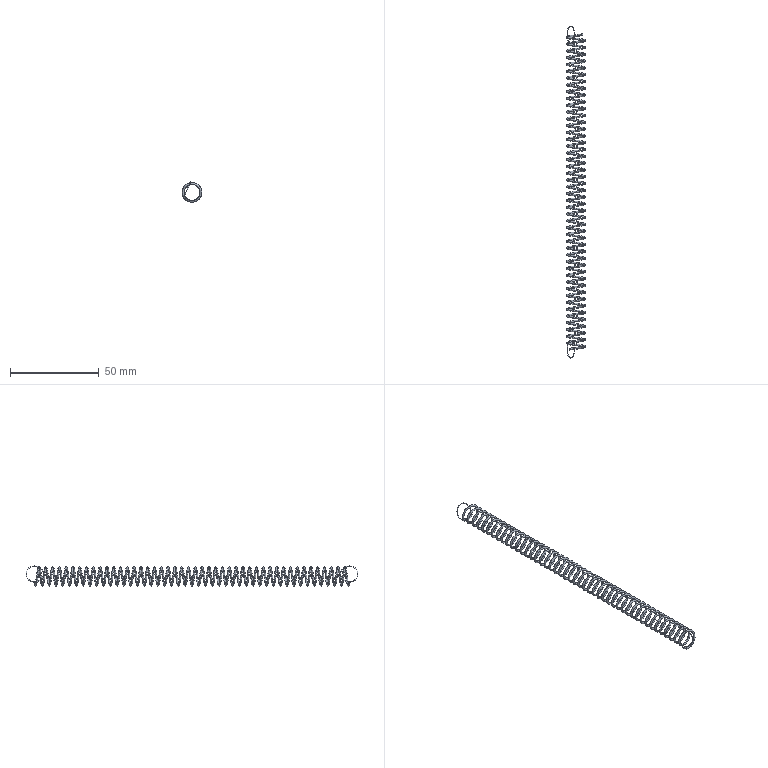Part | SolidWorks | features Helix 1, ICE 1, MirrorSolid 1, Sweep 1 | 3 solids | 16 faces | box 10.978 x 187.418 x 11.39 mm | volume 1153 mm3 | cylinder 8 | plane 6 | spline 2 | commonest cylinder face diameters 9.6 x4 10 x4